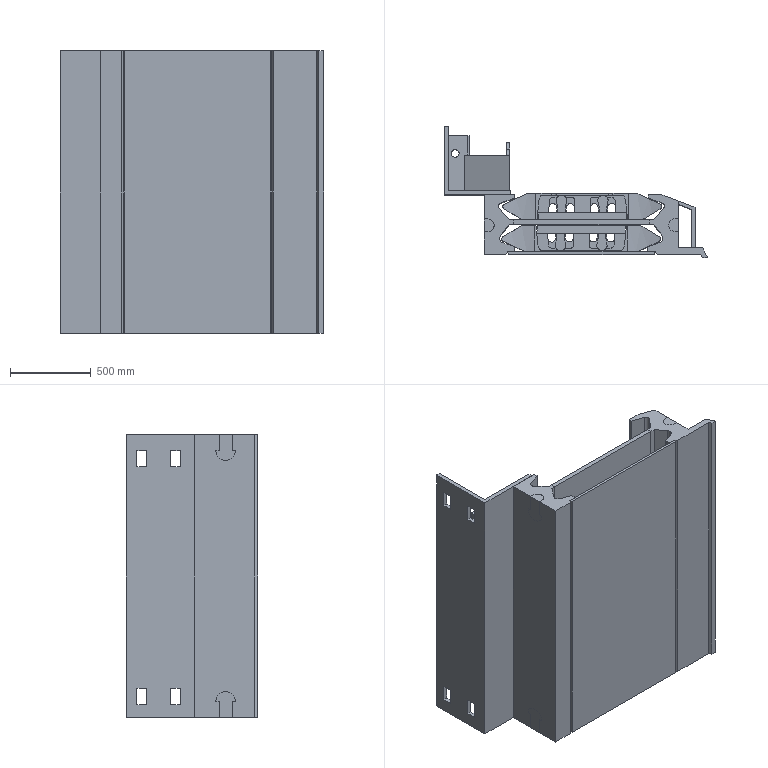Part | SolidWorks | 27 solids | 848 faces | box 1628 x 811.488 x 1750 mm | volume 345627340 mm3 | plane 472 | cylinder 152 | spline 120 | cone 72 | torus 24 | sphere 8 | commonest cylinder face diameters 10 x48 80 x26 70 x14 25 x12 33 x12 50 x12